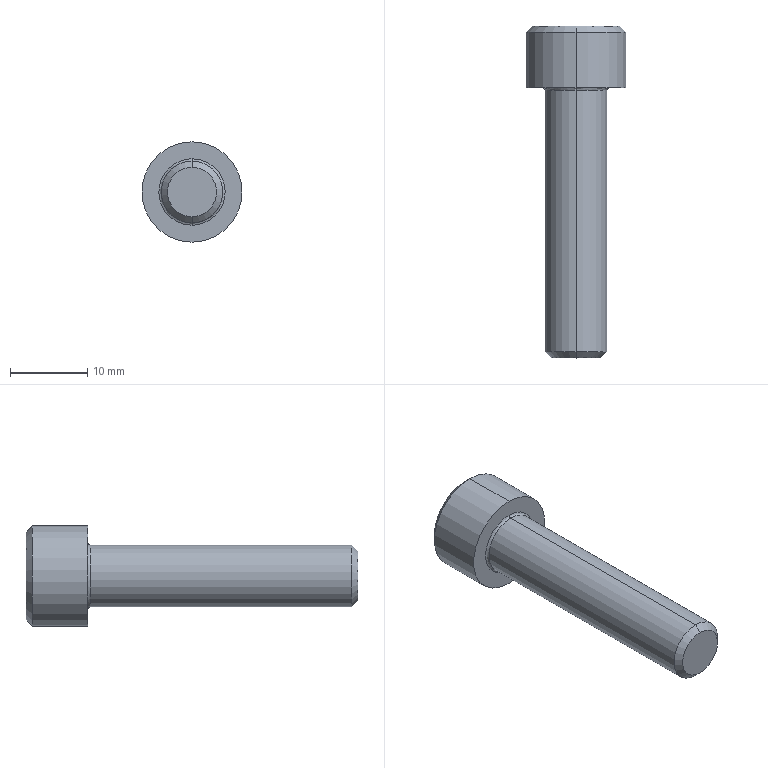Part | STEP file | 1 solid | 20 faces | box 13 x 43 x 13 mm | volume 2615 mm3 | plane 10 | cone 4 | cylinder 4 | spline 2 | commonest cylinder face diameters 8 x2 13 x2